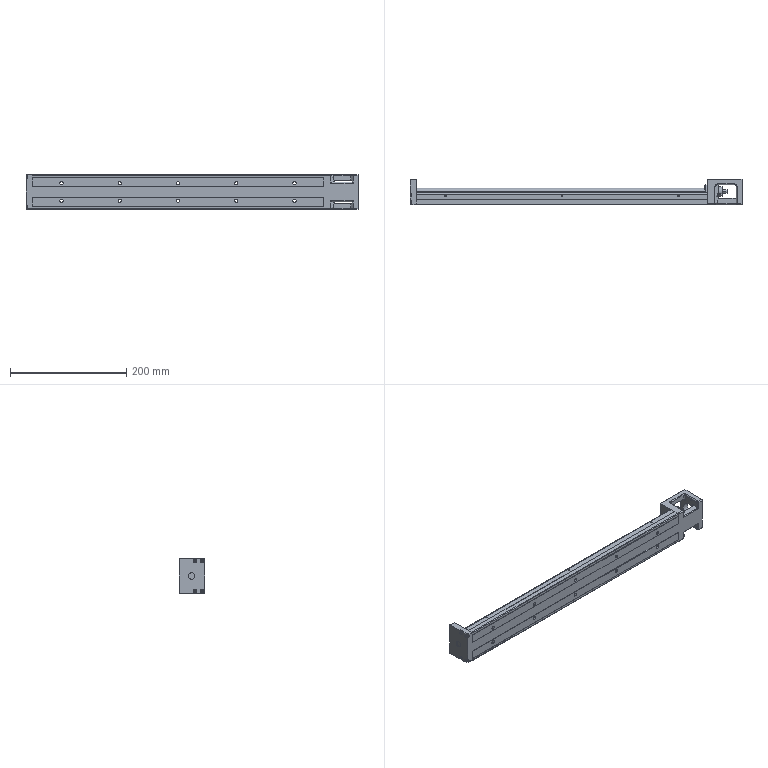Part | STEP file | ASND-0110-KK60-500 | 1 solid | 425 faces | box 570 x 44.5 x 60 mm | volume 511648 mm3 | plane 211 | cylinder 173 | cone 26 | torus 11 | sphere 4 | commonest cylinder face diameters 5.5 x36 3 x27 9.5 x20 3.3 x16 6 x16 2.15 x12